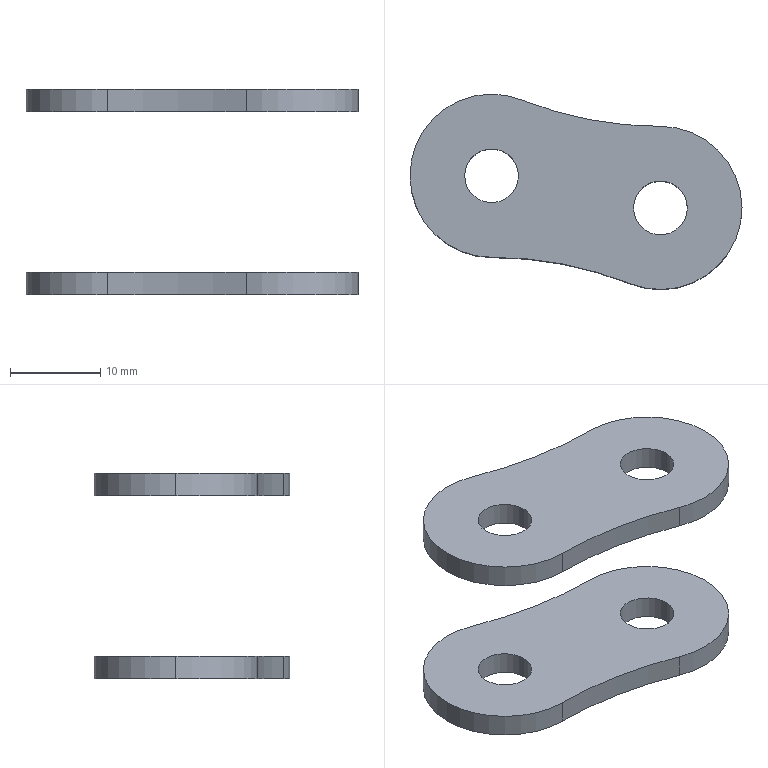Part | STEP file | 2 solids | 22 faces | box 36.793 x 21.646 x 22.78 mm | volume 2638 mm3 | cylinder 18 | plane 4 | commonest cylinder face diameters 5.96 x8 18.08 x6 83.184 x4